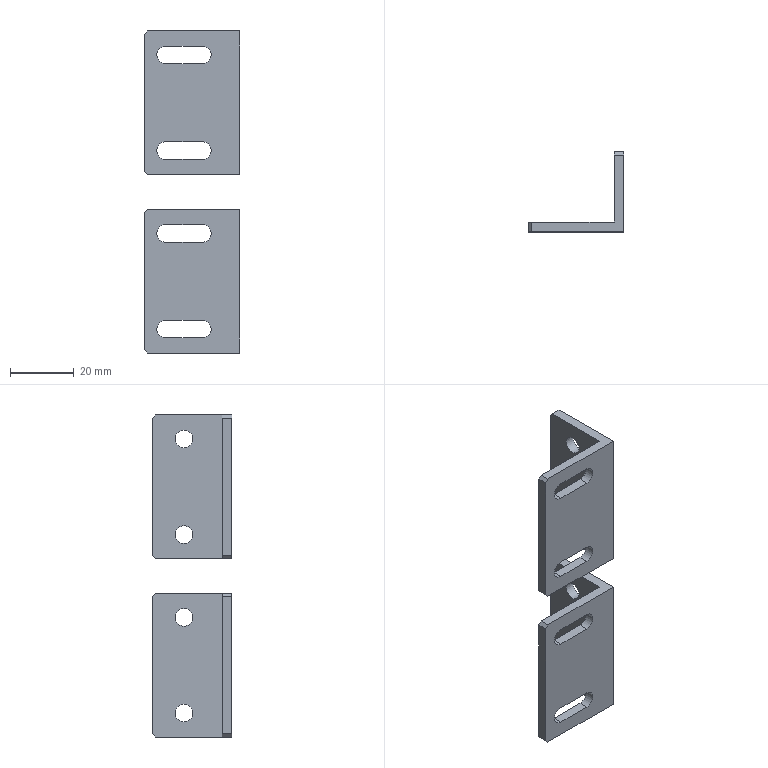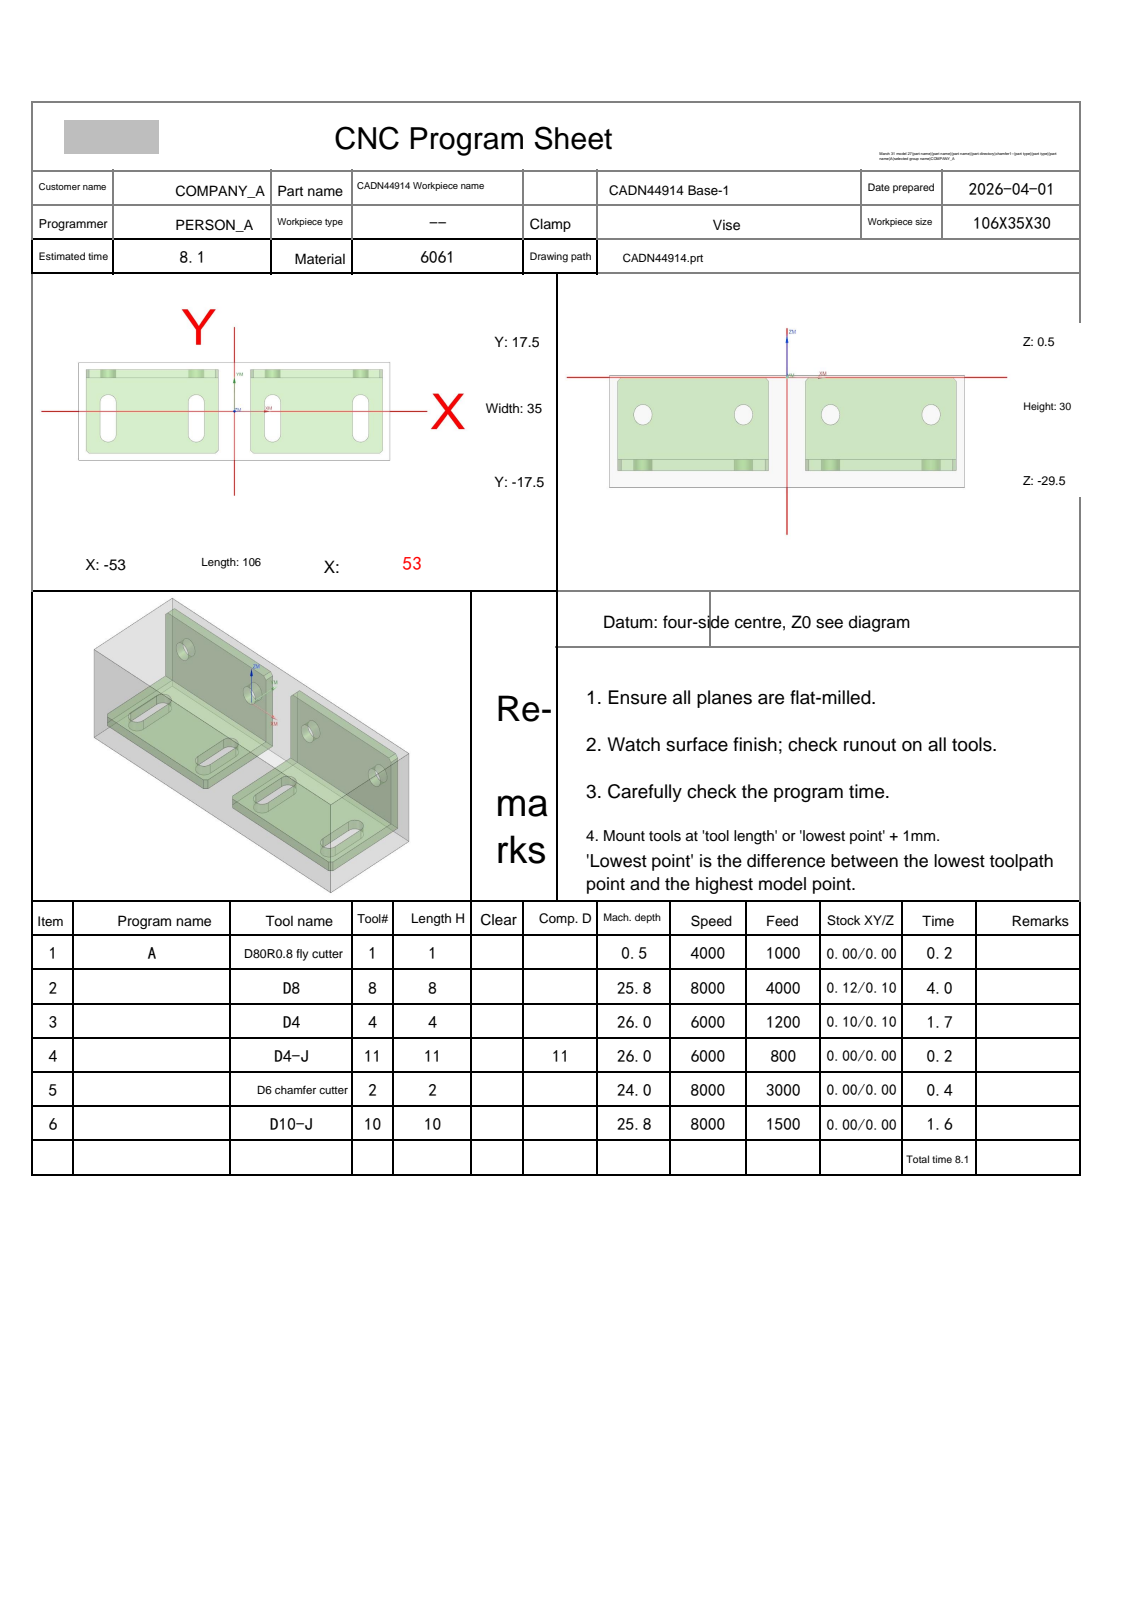NC program | NX | posted by the shop | part box 30 x 25 x 101 mm
Lines 33 to 938 of 5910:
N2 T08 M06
(D8  D=8. R=0. H=08 ce=0.12 di=0.10)
G00 G90 G54 X62.516 Y16.107 M03 S8000
G43 H08 Z20.
M08
Z-10.65
G01 X62.417 Y16.091 Z-11.275 F4000.
X62.318 Y16.075 Z-11.522
X62.219 Y16.059 Z-11.704
X62.121 Y16.043 Z-11.85
X62.022 Y16.027 Z-11.973
X61.923 Y16.011 Z-12.078
X61.825 Y15.995 Z-12.17
X61.726 Y15.979 Z-12.25
X61.627 Y15.963 Z-12.32
X61.529 Y15.947 Z-12.382
X61.43 Y15.931 Z-12.436
X61.331 Y15.915 Z-12.483
X61.232 Y15.899 Z-12.524
X61.134 Y15.883 Z-12.558
X61.035 Y15.867 Z-12.586
X60.936 Y15.851 Z-12.61
X60.838 Y15.835 Z-12.627
X60.739 Y15.819 Z-12.64
X60.64 Y15.803 Z-12.647
X60.541 Y15.787 Z-12.65
X58.872 Y15.515
G03 X58.558 Y15.255 I.069 J-.404
X58.044 Y11.824 I11.196 J-3.431
G01 Y11.754
G03 X57.949 Y3.73 I339.384 J-8.023
X57.95 Y2.791 I339.479 J0.0
G01 X57.931 Y-16.168
G02 X53.968 Y-21.494 I-5.735 J.13
X48.72 Y-22.354 I-5.366 J16.303
X40.208 Y-22.456 I-8.512 J354.954
X38.161 Y-22.45 I0.0 J355.056
G01 X-51.678 Y-22.43
G02 X-56.969 Y-18.509 I.136 J5.714
X-57.846 Y-13.325 I15.967 J5.368
X-57.953 Y-5.477 I289.574 J7.847
X-57.949 Y-4.086 I289.681 J0.0
G01 X-57.931 Y16.154
G02 X-54.076 Y21.44 I5.698 J-.107
X-48.897 Y22.342 I5.375 J-15.529
X-40.524 Y22.458 I8.373 J-302.172
X-38.219 Y22.45 I0.0 J-302.288
G01 X51.741 Y22.427
G02 X57.07 Y18.146 I-.192 J-5.697
X57.491 Y14.544 I-15.208 J-3.602
X57.463 Y13.62 I-15.628 J0.0
G03 X57.351 Y3.991 I606.655 J-11.894
G01 X57.332 Y-14.688
G02 X53.425 Y-20.418 I-6.439 J.194
X47.956 Y-21.66 I-6.092 J14.165
X40.512 Y-21.856 I-7.444 J140.749
X38.96 Y-21.848 I0.0 J140.945
G01 X-50.327 Y-21.825
G02 X-55.877 Y-17.993 I.331 J6.415
X-57.152 Y-12.533 I13.846 J6.11
X-57.358 Y-4.985 I137.85 J7.548
X-57.348 Y-3.297 I138.056 J0.0
G01 X-57.334 Y14.627
G02 X-53.521 Y20.363 I6.425 J-.136
X-47.945 Y21.659 I6.167 J-13.892
X-40.439 Y21.857 I7.506 J-141.907
X-38.829 Y21.848 I0.0 J-142.105
G01 X50.187 Y21.832
G02 X55.925 Y17.551 I-.143 J-6.177
X56.733 Y12.44 I-15.748 J-5.11
G01 Y12.296
G02 X56.763 Y5.932 I-660.189 J-6.364
X56.751 Y1.891 I-660.22 J0.0
X56.771 Y-3.975 I-877.532 J-5.866
X56.718 Y-13.548 I-877.551 J0.0
X52.464 Y-19.656 I-7.15 J.444
X46.419 Y-21.046 I-6.699 J15.305
X38.343 Y-21.259 I-8.076 J152.558
X36.463 Y-21.248 I0.0 J152.772
G01 X-48.937 Y-21.224
G02 X-55.152 Y-16.964 I.346 J7.169
X-56.53 Y-11.098 I15.026 J6.624
X-56.762 Y-2.879 I145.33 J8.219
X-56.748 Y-.843 I145.562 J0.0
X-56.767 Y4.609 I770.486 J5.452
X-56.715 Y13.577 I770.505 J0.0
X-52.493 Y19.637 I7.146 J-.478
X-46.749 Y21.017 I6.58 J-14.744
X-38.468 Y21.264 I8.281 J-138.804
X-36.375 Y21.248 I0.0 J-139.051
G01 X48.785 Y21.231
G02 X54.926 Y16.953 I-.153 J-6.766
X56.047 Y11.274 I-15.235 J-5.957
X56.174 Y1.718 I-357.138 J-9.556
X56.15 Y-2.427 I-357.266 J0.0
X56.174 Y-6.04 I-275.832 J-3.613
X56.099 Y-12.466 I-275.856 J0.0
X51.293 Y-19.07 I-7.778 J.609
X44.934 Y-20.447 I-7.048 J17.185
X36.468 Y-20.659 I-8.466 J168.493
X34.498 Y-20.648 I0.0 J168.706
G01 X-47.542 Y-20.626
G02 X-54.546 Y-15.835 I.2 J7.809
X-55.919 Y-9.777 I16.529 J6.929
X-56.163 Y-1.075 I154.575 J8.702
X-56.148 Y1.138 I154.819 J0.0
X-56.157 Y4.648 I663.047 J3.51
X-56.113 Y12.257 I663.056 J0.0
X-53.836 Y17.363 I7.476 J-.274
X-51.867 Y18.926 I3.623 J-2.541
X-45.235 Y20.432 I7.404 J-17.255
X-36.921 Y20.657 I8.314 J-153.529
X-35.159 Y20.647 I0.0 J-153.754
G01 X47.421 Y20.631
G02 X52.399 Y18.635 I-.044 J-7.317
X54.068 Y17.06 I-2.112 J-3.911
X55.259 Y12.19 I-13.92 J-5.984
X55.559 Y4.973 I-86.472 J-7.217
X55.547 Y3.499 I-86.773 J0.0
X55.566 Y-2.101 I-811.454 J-5.6
X55.518 Y-10.94 I-811.473 J0.0
X50.295 Y-18.445 I-8.318 J.219
X43.928 Y-19.823 I-7.236 J18.035
X35.476 Y-20.056 I-8.452 J153.016
X33.732 Y-20.046 I0.0 J153.249
G01 X-46.027 Y-20.034
X-46.181 Y-20.035
G02 X-53.946 Y-14.785 I0.0 J8.368
X-55.34 Y-8.184 I18.432 J7.341
X-55.554 Y.16 I162.754 J8.345
X-55.546 Y1.772 I162.968 J0.0
X-55.57 Y5.167 I243.213 J3.395
X-55.493 Y11.271 I243.237 J0.0
X-54.62 Y14.627 I10.704 J-.994
X-54.625 Y14.848 I4.478 J.221
X-53.413 Y17.913 I4.483 J0.0
X-50.498 Y19.12 I3.041 J-3.221
X-38.847 Y20.04 I11.651 J-73.341
X-37.813 Y20.032 I0.0 J-74.261
G01 X46.087 Y20.031
G02 X49.997 Y19.12 I-.377 J-10.464
X50.293 Y19.129 I.296 J-4.764
X52.453 Y18.612 I0.0 J-4.773
G03 X50.253 Y19.134 I-2.2 J-4.376
X49.877 Y19.12 I0.0 J-4.898
X42.529 Y19.577 I-7.348 J-58.761
X41.176 Y19.562 I0.0 J-59.218
G01 X-38.344 Y19.543
X-38.43
G03 X-46.798 Y19.12 I0.0 J-82.957
G01 X-50.498
X-5.206 Y19.099
G03 X2.028 Y18.963 I7.233 J191.611
X4.429 Y18.978 I0.0 J191.748
G01 X5.502 Y19.12
X49.902
G03 X50.302 Y19.52 I0.0 J.4
X50.116 Y19.857 I-.4 J0.0
G01 X49.518 Y20.237
X48.185 Y21.084 Z-12.55
X47.915 Y21.255
X47.866 Y21.282
X47.814 Y21.301
X47.759 Y21.313
X47.704 Y21.318
X5.983 Y21.67
X5.917 Y21.665
X5.852 Y21.648
X5.79 Y21.622
X5.734 Y21.585
X5.685 Y21.54
X5.644 Y21.487
X5.613 Y21.428
X5.478 Y21.116
X4.85 Y19.667 Z-12.65
X4.727 Y19.37
G02 X4.038 Y18.853 I-.713 J.232
X-.04 Y18.522 I-4.078 J24.962
X-.806 Y18.534 I0.0 J25.293
G01 X-3.48 Y18.584
G03 X-5.498 Y19.12 I-2.169 J-4.106
G02 X-3.387 Y18.54 I-.174 J-4.768
G03 X-.092 Y18.042 I3.295 J10.652
X.316 Y18.049 I0.0 J11.151
X.604 Y18.047 I.288 J17.386
X2.942 Y18.205 I0.0 J17.389
G02 X4.327 Y18.935 I2.618 J-3.285
G03 X2.916 Y18.173 I1.146 J-3.809
G02 X.092 Y17.684 I-2.824 J7.906
X-.583 Y17.711 I0.0 J8.396
X-2.733 Y18.025 I.065 J7.962
G01 X-3.44 Y18.568
G03 X-.35 Y17.337 I3.115 J3.325
X.324 Y17.304 I.674 J6.969
X2.291 Y17.586 I0.0 J7.002
G02 X2.968 Y18.205 I3.756 J-3.425
G03 X2.327 Y17.586 I1.262 J-1.946
G02 X.075 Y17.02 I-2.252 J4.193
X-.563 Y17.063 I0.0 J4.76
X-2.302 Y17.542 I.006 J3.412
G01 X-2.634 Y17.95
G03 X-.588 Y16.782 I2.21 J1.496
X.191 Y16.712 I.778 J4.275
X1.92 Y17.071 I0.0 J4.345
G01 X2.385 Y17.65
G02 X.59 Y16.541 I-1.891 J1.053
X-.018 Y16.491 I-.608 J3.719
X-1.862 Y16.973 I0.0 J3.769
G01 X-2.268 Y17.498
G03 X-.107 Y16.241 I2.161 J1.229
G01 X-.033 Y16.242
G03 X.291 Y16.221 I.324 J2.437
X1.776 Y16.72 I0.0 J2.458
G01 X1.932 Y17.06
G02 X.952 Y16.188 I-1.2 J.361
X.024 Y16.034 I-.928 J2.735
X-1.732 Y16.629 I0.0 J2.889
G01 X-1.932 Y17.06
G03 X-.503 Y15.885 I1.602 J.492
X.117 Y15.807 I.62 J2.416
X1.586 Y16.285 I0.0 J2.494
G01 X1.809 Y16.763
G02 X.631 Y15.724 I-1.342 J.335
X-.008 Y15.634 I-.639 J2.23
X-1.597 Y16.264 I0.0 J2.32
G01 X-1.773 Y16.676
G03 X-.166 Y15.461 I1.621 J.474
X.163 Y15.433 I.329 J1.919
X1.459 Y15.928 I0.0 J1.947
G01 X1.635 Y16.343
G02 X.509 Y15.351 I-1.257 J.292
X.006 Y15.291 I-.503 J2.051
X-1.45 Y15.873 I0.0 J2.112
G01 X-1.612 Y16.288
G03 X-.263 Y15.14 I1.426 J.309
X.141 Y15.091 I.404 J1.643
X1.456 Y15.718 I0.0 J1.692
G01 X1.52 Y16.066
G02 X.681 Y15.084 I-1.026 J.027
X.015 Y14.964 I-.666 J1.788
X-1.436 Y15.632 I0.0 J1.908
G01 X-1.51 Y15.99
G03 X-.594 Y14.908 I1.164 J.056
X.061 Y14.785 I.655 J1.688
X1.392 Y15.368 I0.0 J1.81
G01 X1.493 Y15.862
X1.494 Y15.834
G02 X.546 Y14.739 I-1.106 J0.0
X.009 Y14.657 I-.537 J1.711
X-1.403 Y15.344 I0.0 J1.793
G01 X-1.478 Y15.743
G03 X-.419 Y14.558 I1.224 J.029
X.085 Y14.479 I.504 J1.563
X1.376 Y15.106 I0.0 J1.642
G01 X1.452 Y15.549
X1.453 Y15.526
G02 X.494 Y14.431 I-1.105 J0.0
X-.016 Y14.349 I-.51 J1.538
X-1.388 Y15.107 I0.0 J1.621
G01 X-1.438 Y15.438
G03 X-.425 Y14.269 I1.205 J.021
X.067 Y14.194 I.492 J1.563
X1.334 Y14.794 I0.0 J1.639
G01 X1.412 Y15.239
Y15.205
G02 X.497 Y14.147 I-1.07 J0.0
X.004 Y14.071 I-.492 J1.556
X-1.351 Y14.794 I0.0 J1.632
G01 X-1.396 Y15.119
Y15.103
G03 X-.521 Y14.021 I1.106 J0.0
X.068 Y13.904 I.59 J1.428
X1.356 Y14.595 I0.0 J1.545
G01 X1.38 Y15.001
X1.391 Y14.861
G02 X.67 Y13.931 I-.961 J0.0
X.009 Y13.786 I-.661 J1.438
X-1.365 Y14.583 I0.0 J1.583
G01 X-1.38 Y14.906
X-1.385 Y14.804
G03 X-.551 Y13.755 I1.076 J0.0
X.057 Y13.633 I.609 J1.458
X1.349 Y14.304 I0.0 J1.58
G01 X1.381 Y14.678
X1.386 Y14.573
G02 X.685 Y13.661 I-.944 J0.0
X.014 Y13.512 I-.671 J1.437
X-1.365 Y14.314 I0.0 J1.586
G01 X-1.381 Y14.638
X-1.385 Y14.537
G03 X-.537 Y13.475 I1.088 J0.0
X.066 Y13.352 I.603 J1.414
X1.358 Y14.057 I0.0 J1.537
G01 X1.381 Y14.404
X1.386 Y14.305
G02 X.682 Y13.385 I-.953 J0.0
X.016 Y13.239 I-.667 J1.449
X-1.363 Y14.032 I0.0 J1.595
G01 X-1.381 Y14.364
X-1.386 Y14.261
G03 X-.565 Y13.211 I1.082 J0.0
X.057 Y13.081 I.622 J1.432
X1.355 Y13.775 I0.0 J1.561
G01 X1.381 Y14.198
X1.393 Y14.044
G02 X.699 Y13.118 I-.965 J0.0
X.018 Y12.967 I-.681 J1.465
X-1.356 Y13.733 I0.0 J1.616
G01 X-1.382 Y14.095
X-1.387 Y13.989
G03 X-.567 Y12.936 I1.086 J0.0
X.067 Y12.799 I.633 J1.393
X1.361 Y13.514 I0.0 J1.53
G01 X1.381 Y13.852
X1.387 Y13.752
G02 X.7 Y12.843 I-.944 J0.0
X.011 Y12.684 I-.689 J1.417
X-1.368 Y13.497 I0.0 J1.575
G01 X-1.382 Y13.815
X-1.387 Y13.711
G03 X-.567 Y12.661 I1.082 J0.0
X.053 Y12.536 I.619 J1.474
X1.344 Y13.193 I0.0 J1.599
G01 X1.382 Y13.58
X1.387 Y13.48
G02 X.682 Y12.561 I-.951 J0.0
X.015 Y12.416 I-.667 J1.455
X-1.362 Y13.201 I0.0 J1.6
G01 X-1.382 Y13.54
X-1.387 Y13.439
G03 X-.547 Y12.379 I1.088 J0.0
X.064 Y12.253 I.611 J1.412
X1.36 Y12.963 I0.0 J1.538
G01 X1.382 Y13.308
X1.387 Y13.21
G02 X.682 Y12.286 I-.957 J0.0
X.014 Y12.14 I-.667 J1.445
X-1.366 Y12.937 I0.0 J1.592
G01 X-1.383 Y13.267
X-1.388 Y13.162
G03 X-.566 Y12.111 I1.083 J0.0
X.052 Y11.987 I.619 J1.474
X1.346 Y12.647 I0.0 J1.598
G01 X1.382 Y13.091
X1.393 Y12.949
G02 X.682 Y12.012 I-.972 J0.0
X.014 Y11.866 I-.667 J1.452
X-1.364 Y12.655 I0.0 J1.598
G01 X-1.383 Y12.992
X-1.388 Y12.888
G03 X-.567 Y11.836 I1.084 J0.0
X.053 Y11.71 I.62 J1.461
X1.35 Y12.382 I0.0 J1.587
G01 X1.383 Y12.818
X1.393 Y12.675
G02 X.682 Y11.737 I-.973 J0.0
X.014 Y11.591 I-.668 J1.448
X-1.363 Y12.381 I0.0 J1.595
G01 X-1.384 Y12.721
X-1.389 Y12.614
G03 X-.582 Y11.567 I1.084 J0.0
X.063 Y11.425 I.644 J1.395
X1.362 Y12.142 I0.0 J1.536
G01 X1.383 Y12.542
X1.393 Y12.4
G02 X.685 Y11.462 I-.975 J0.0
X.015 Y11.315 I-.67 J1.452
X-1.365 Y12.106 I0.0 J1.599
G01 X-1.384 Y12.443
X-1.389 Y12.34
G03 X-.57 Y11.285 I1.09 J0.0
X.049 Y11.16 I.619 J1.482
X1.345 Y11.819 I0.0 J1.606
G01 X1.383 Y12.266
X1.392 Y12.132
G02 X.639 Y11.164 I-.998 J0.0
X.019 Y11.04 I-.62 J1.488
X-1.36 Y11.817 I0.0 J1.612
G01 X-1.385 Y12.178
X-1.39 Y12.067
G03 X-.582 Y11.014 I1.089 J0.0
X.062 Y10.871 I.644 J1.379
X1.376 Y11.625 I0.0 J1.522
G01 X1.383 Y12.011
X1.396 Y11.852
G02 X.653 Y10.894 I-.989 J0.0
X.015 Y10.759 I-.638 J1.451
X-1.38 Y11.591 I0.0 J1.585
G01 X-1.385 Y11.908
X-1.395 Y11.765
G03 X-.67 Y10.775 I1.039 J0.0
X.052 Y10.598 I.723 J1.39
X1.42 Y11.4 I0.0 J1.567
G01 X1.386 Y11.818
G02 X1.429 Y11.544 I-.848 J-.274
X.867 Y10.716 I-.891 J0.0
X.024 Y10.474 I-.843 J1.351
X-1.43 Y11.418 I0.0 J1.592
G01 X-1.397 Y11.73
G03 X-1.433 Y11.473 I.921 J-.257
X-.885 Y10.608 I.956 J0.0
X.042 Y10.319 I.927 J1.34
X1.466 Y11.156 I0.0 J1.63
X1.434 Y11.577 I-3.694 J-.073
G02 X1.477 Y11.299 I-.873 J-.278
X.915 Y10.453 I-.917 J0.0
X.03 Y10.199 I-.885 J1.41
X-1.47 Y11.144 I0.0 J1.664
G01 X-1.445 Y11.501
G03 X-1.481 Y11.234 I.953 J-.268
X-.949 Y10.356 I.99 J0.0
X.041 Y10.036 I.991 J1.373
X1.51 Y10.887 I0.0 J1.693
G01 X1.513 Y10.99
G03 X1.484 Y11.32 I-1.88 J0.0
G02 X1.524 Y11.047 I-.903 J-.273
X.967 Y10.186 I-.943 J0.0
X.032 Y9.907 I-.935 J1.428
X-1.525 Y10.914 I0.0 J1.707
G01 X-1.485 Y11.306
G03 X-1.531 Y10.994 I1.023 J-.311
X-.896 Y10.017 I1.069 J0.0
X.045 Y9.738 I.941 J1.447
X1.567 Y10.651 I0.0 J1.726
X1.522 Y11.127 I-3.127 J-.059
G02 X1.58 Y10.796 I-.912 J-.332
X1.052 Y9.932 I-.97 J0.0
X.033 Y9.607 I-1.019 J1.437
X-1.583 Y10.665 I0.0 J1.762
G01 X-1.539 Y11.042
G03 X-1.586 Y10.726 I1.038 J-.316
X-.951 Y9.738 I1.085 J0.0
X.046 Y9.434 I.997 J1.481
X1.621 Y10.379 I0.0 J1.786
X1.58 Y10.832 I-3.737 J-.111
G02 X1.635 Y10.513 I-.9 J-.32
X1.156 Y9.685 I-.955 J0.0
X.034 Y9.299 I-1.123 J1.44
X-1.639 Y10.392 I0.0 J1.826
G01 X-1.601 Y10.743
G03 X-1.637 Y10.461 I1.097 J-.282
X-.977 Y9.431 I1.133 J0.0
X.047 Y9.121 I1.025 J1.534
X1.686 Y10.117 I0.0 J1.845
G01 X1.714 Y10.294
G03 X1.626 Y10.597 I-.569 J0.0
G02 X1.73 Y10.21 I-.671 J-.387
X1.459 Y9.621 I-.775 J0.0
X.039 Y8.981 I-1.42 J1.255
X-1.695 Y10.11 I0.0 J1.895
G01 X-1.717 Y10.27
G02 X-1.637 Y10.566 I.593 J0.0
G03 X-1.746 Y10.147 I.755 J-.419
X-1.475 Y9.519 I.864 J0.0
X.043 Y8.804 I1.519 J1.255
X1.744 Y9.78 I0.0 J1.97
X1.826 Y10.093 I-.557 J.314
X1.678 Y10.503 I-.639 J0.0
G02 X1.841 Y9.99 I-.724 J-.513
X1.524 Y9.31 I-.888 J0.0
X.04 Y8.662 I-1.485 J1.376
X-1.735 Y9.713 I0.0 J2.024
X-1.825 Y10.055 I.605 J.343
X-1.702 Y10.451 I.696 J0.0
G03 X-1.858 Y9.921 I.817 J-.53
X-1.56 Y9.22 I.974 J0.0
X.046 Y8.468 I1.606 J1.34
X1.843 Y9.488 I0.0 J2.092
X1.946 Y9.862 I-.623 J.374
X1.766 Y10.341 I-.726 J0.0
G02 X1.966 Y9.757 I-.753 J-.584
X1.668 Y9.064 I-.953 J0.0
X.043 Y8.315 I-1.624 J1.387
X-1.865 Y9.492 I0.0 J2.136
X-1.948 Y9.833 I.66 J.341
X-1.793 Y10.287 I.743 J0.0
G03 X-1.979 Y9.677 I.91 J-.61
X-1.611 Y8.858 I1.096 J0.0
X.049 Y8.113 I1.66 J1.478
X1.974 Y9.226 I0.0 J2.223
X2.08 Y9.601 I-.613 J.375
X1.932 Y10.038 I-.719 J0.0
G02 X2.1 Y9.488 I-.812 J-.55
X1.818 Y8.8 I-.981 J0.0
X.049 Y7.946 I-1.769 J1.407
X-2.022 Y9.301 I0.0 J2.26
X-2.081 Y9.592 I.695 J.291
X-1.921 Y10.056 I.754 J0.0
G03 X-2.118 Y9.418 I.935 J-.638
X-1.799 Y8.63 I1.132 J0.0
X.051 Y7.74 I1.85 J1.476
X2.113 Y8.944 I0.0 J2.367
X2.222 Y9.34 I-.661 J.396
X2.045 Y9.831 I-.771 J0.0
G02 X2.245 Y9.221 I-.83 J-.611
X1.974 Y8.524 I-1.031 J0.0
X.048 Y7.568 I-1.927 J1.462
X-2.142 Y8.959 I0.0 J2.418
X-2.224 Y9.32 I.746 J.361
X-2.041 Y9.84 I.829 J0.0
G03 X-2.266 Y9.145 I.963 J-.695
X-1.95 Y8.338 I1.188 J0.0
X.053 Y7.345 I2.003 J1.525
X2.262 Y8.655 I0.0 J2.518
X2.378 Y9.067 I-.674 J.412
X2.171 Y9.601 I-.79 J0.0
G02 X2.417 Y8.957 I-.721 J-.644
X2.248 Y8.41 I-.967 J0.0
X.041 Y7.176 I-2.207 J1.356
X-2.261 Y8.579 I0.0 J2.59
X-2.383 Y9.019 I.734 J.44
X-2.214 Y9.529 I.856 J0.0
G03 X-2.449 Y8.88 I.778 J-.649
X-2.292 Y8.338 I1.013 J0.0
X.068 Y6.939 I2.361 J1.291
X2.407 Y8.299 I0.0 J2.69
X2.558 Y8.821 I-.825 J.523
X2.434 Y9.299 I-.977 J0.0
G01 X2.261 Y9.465
G02 X2.621 Y8.722 I-.586 J-.743
X2.491 Y8.244 I-.946 J0.0
X.059 Y6.747 I-2.433 J1.229
X-1.039 Y6.978 I0.0 J2.725
X-2.552 Y8.88 I.688 J2.1
G01 Y8.903
G02 X-2.248 Y9.472 I.685 J0.0
G03 X-2.651 Y8.646 I.644 J-.826
X-2.53 Y8.156 I1.047 J0.0
X.059 Y6.501 I2.589 J1.196
X1.116 Y6.704 I0.0 J2.852
X2.761 Y8.695 I-.636 J2.201
X2.415 Y9.317 I-.729 J0.0
G02 X2.839 Y8.494 I-.587 J-.823
X2.74 Y8.058 I-1.011 J0.0
X.127 Y6.312 I-2.614 J1.084
X-.37 Y6.356 I0.0 J2.83
X-2.746 Y8.412 I.215 J2.649
X-2.772 Y8.62 I.815 J.208
X-2.44 Y9.29 I.841 J0.0
G03 X-2.871 Y8.399 I.705 J-.89
X-2.768 Y7.927 I1.135 J0.0
X.026 Y6.05 I2.795 J1.141
X.766 Y6.142 I0.0 J3.019
X2.988 Y8.316 I-.394 J2.625
G01 X3. Y8.449
G03 X2.643 Y9.098 I-.769 J0.0
G02 X3.078 Y8.247 I-.614 J-.851
X3.008 Y7.869 I-1.05 J0.0
X.204 Y5.863 I-2.803 J.956
G01 X.104 Y5.865
X-.074 Y5.86
G02 X-2.94 Y7.955 I0.0 J3.009
X-3.009 Y8.321 I.942 J.366
X-2.625 Y9.114 I1.01 J0.0
G03 X-3.111 Y8.141 I.732 J-.973
X-3.023 Y7.688 I1.218 J0.0
X-.025 Y5.583 I2.999 J1.083
X.354 Y5.605 I0.0 J3.188
X3.209 Y7.822 I-.073 J3.041
X3.259 Y8.123 I-.871 J.302
X2.89 Y8.861 I-.922 J0.0
G02 X3.336 Y7.947 I-.713 J-.914
X3.241 Y7.487 I-1.159 J0.0
X.195 Y5.37 I-3.046 J1.134
X-.044 Y5.379 I0.0 J3.25
G01 X-.094
G02 X-3.185 Y7.647 I0.0 J3.241
X-3.246 Y8.043 I1.265 J.395
X-3.083 Y8.679 I1.325 J0.0
G01 X-2.866 Y8.885
G03 X-3.369 Y7.844 I.826 J-1.041
X-3.264 Y7.329 I1.329 J0.0
X-.051 Y5.09 I3.214 J1.187
G01 X.119 Y5.094
X.233 Y5.092
G03 X3.425 Y7.31 I0.0 J3.405
X3.528 Y7.806 I-1.136 J.496
X3.292 Y8.534 I-1.239 J0.0
G01 X3.134 Y8.627
G02 X3.604 Y7.873 I-.37 J-.753
G01 X3.598 Y7.772
G02 X1.749 Y5.233 I-2.932 J.193
X.071 Y4.845 I-1.679 J3.438
X-3.236 Y6.747 I0.0 J3.826
X-3.508 Y7.69 I1.498 J.943
X-3.31 Y8.503 I1.77 J0.0
G01 X-3.148 Y8.618
G03 X-3.636 Y7.791 I.456 J-.827
G01 X-3.63 Y7.684
G03 X-1.725 Y4.98 I3.091 J.154
X.087 Y4.544 I1.812 J3.551
X3.524 Y6.511 I0.0 J3.986
X3.802 Y7.502 I-1.621 J.991
X3.6 Y8.355 I-1.9 J0.0
G01 X3.217 Y8.586
G02 X3.914 Y7.621 I-.319 J-.965
G01 X3.907 Y7.505
G02 X1.97 Y4.766 I-3.178 J.193
X.079 Y4.312 I-1.891 J3.714
X-3.442 Y6.249 I0.0 J4.168
X-3.795 Y7.406 I1.718 J1.157
X-3.554 Y8.377 I2.072 J0.0
G01 X-3.224 Y8.58
G03 X-3.94 Y7.548 I.386 J-1.032
G01 X-3.939 Y7.499
G03 X-2.037 Y4.549 I3.298 J.038
X.082 Y4. I2.119 J3.817
X3.726 Y5.961 I0.0 J4.366
X4.125 Y7.237 I-1.84 J1.276
X3.915 Y8.183 I-2.239 J0.0
X3.452 Y8.47 I-1.292 J-1.568
G02 X4.256 Y7.36 I-.365 J-1.11
G01 X4.247 Y7.214
G02 X2.177 Y4.266 I-3.47 J.236
X.083 Y3.75 I-2.094 J3.989
X-3.754 Y5.893 I0.0 J4.506
X-4.12 Y7.134 I1.916 J1.24
X-3.837 Y8.235 I2.283 J0.0
G01 X-3.448 Y8.47
G03 X-4.293 Y7.246 I.465 J-1.224
G01 X-4.284 Y7.09
G03 X-2.123 Y3.976 I3.664 J.236
X.086 Y3.43 I2.21 J4.195
X4.018 Y5.521 I0.0 J4.741
X4.477 Y6.97 I-2.058 J1.449
X4.25 Y8.013 I-2.517 J0.0
X3.784 Y8.306 I-1.157 J-1.326
G02 X4.614 Y7.146 I-.395 J-1.159
G01 X4.611 Y7.059
G02 X2.579 Y3.843 I-3.695 J.084
X.094 Y3.166 I-2.485 J4.223
X-4.033 Y5.424 I0.0 J4.9
X-4.47 Y6.858 I2.132 J1.434
X-4.176 Y8.051 I2.569 J0.0
X-3.763 Y8.316 I1.173 J-1.376
G03 X-4.636 Y7.063 I.463 J-1.253
G01 Y7.052
X-4.638 Y6.935
G03 X-2.863 Y3.759 I3.73 J0.0
X.084 Y2.831 I2.948 J4.216
X4.368 Y5.127 I0.0 J5.144
X4.854 Y6.714 I-2.347 J1.587
X4.672 Y7.715 I-2.833 J0.0
X4.152 Y8.124 I-.697 J-.349
G02 X4.944 Y7.206 I-.267 J-1.03
X4.983 Y6.68 I-3.497 J-.527
X3.686 Y3.942 I-3.536 J0.0
X.105 Y2.564 I-3.581 J3.965
X-4.264 Y4.831 I0.0 J5.343
X-4.839 Y6.59 I2.403 J1.758
X-4.615 Y7.723 I2.977 J0.0
X-4.052 Y8.174 I.819 J-.444
G03 X-5.025 Y6.836 I.446 J-1.347
G01 X-5.029 Y6.654
G03 X-3.2 Y3.285 I4.016 J0.0
X.088 Y2.216 I3.288 J4.523
X4.638 Y4.557 I0.0 J5.592
X5.257 Y6.429 I-2.52 J1.872
X5.055 Y7.536 I-3.139 J0.0
X4.316 Y8.066 I-.739 J-.25
G01 X4.293
G02 X5.291 Y7.221 I-.027 J-1.043
X5.405 Y6.329 I-3.423 J-.892
X4.46 Y3.922 I-3.537 J0.0
X.104 Y1.937 I-4.356 J3.787
X-4.602 Y4.368 I0.0 J5.772
X-5.239 Y6.321 I2.677 J1.953
X-5.048 Y7.431 I3.314 J0.0
X-4.267 Y8.069 I.849 J-.243
G03 X-5.282 Y7.233 I.074 J-1.123
X-5.444 Y6.159 I3.464 J-1.073
X-4.557 Y3.783 I3.627 J0.0
X.104 Y1.578 I4.66 J3.824
X5.002 Y4.093 I0.0 J6.029
X5.689 Y6.18 I-2.828 J2.086
X5.506 Y7.296 I-3.514 J0.0
X4.57 Y8.023 I-.938 J-.242
G01 X4.578
G02 X5.66 Y7.222 I0.0 J-1.132
X5.861 Y6.031 I-3.432 J-1.191
X5.112 Y3.822 I-3.633 J0.0
X.1 Y1.29 I-5.012 J3.696
X-4.936 Y3.854 I0.0 J6.228
X-5.669 Y6.061 I2.955 J2.207
X-5.489 Y7.199 I3.688 J0.0
X-4.812 Y7.986 I1.28 J-.418
G01 X-4.515 Y8.031
G03 X-5.745 Y6.987 I.085 J-1.347
X-5.892 Y5.909 I3.887 J-1.078
X-4.858 Y3.212 I4.034 J0.0
X.106 Y.914 I4.964 J4.212
X5.413 Y3.653 I0.0 J6.51
X6.152 Y5.915 I-3.089 J2.262
X5.939 Y7.173 I-3.829 J0.0
X4.949 Y7.965 I-1.029 J-.271
G02 X6.08 Y7.153 I-.009 J-1.207
X6.343 Y5.759 I-3.568 J-1.394
X5.669 Y3.588 I-3.831 J0.0
X.122 Y.615 I-5.547 J3.688
X-2.021 Y.969 I0.0 J6.661
X-6.053 Y5.055 I1.571 J5.583
X-6.164 Y5.855 I2.806 J.8
X-5.474 Y7.74 I2.917 J0.0
X-4.851 Y7.985 I.623 J-.668
G01 X-4.819 Y7.984
G03 X-6.152 Y6.955 I.052 J-1.445
X-6.375 Y5.612 I3.944 J-1.342
X-5.532 Y3.1 I4.166 J0.0
X.125 Y.23 I5.657 J4.139
X3.245 Y.963 I0.0 J7.009
X6.633 Y5.331 I-2.313 J5.291
X6.677 Y5.823 I-2.733 J.492
X5.85 Y7.8 I-2.777 J0.0
X5.32 Y7.908 I-.671 J-1.938
G01 X5.365 Y7.909
G02 X6.515 Y7.117 I0.0 J-1.231
X6.853 Y5.5 I-3.695 J-1.616
X6.266 Y3.405 I-4.033 J0.0
X.208 Y-.066 I-6.058 J3.55
X-.665 Y-.012 I0.0 J7.021
X-6.318 Y4.005 I.495 J6.683
X-6.639 Y5.513 I3.382 J1.508
X-6.135 Y7.377 I3.703 J0.0
X-5.214 Y7.925 I.921 J-.5
G01 X-5.205
G03 X-6.563 Y6.961 I.026 J-1.475
X-6.885 Y5.334 I3.952 J-1.628
X-6.254 Y3.098 I4.274 J0.0
X.027 Y-.463 I6.28 J3.757
X1.094 Y-.385 I0.0 J7.318
X6.835 Y3.791 I-.682 J6.971
X7.184 Y5.398 I-3.527 J1.607
X6.666 Y7.334 I-3.876 J0.0
X5.776 Y7.891 I-.89 J-.432
G01 X5.63 Y7.88
X5.786 Y7.89
G02 X6.937 Y7.143 I0.0 J-1.261
X7.392 Y5.256 I-3.694 J-1.887
X6.96 Y3.413 I-4.148 J0.0
X.71 Y-.738 I-6.605 J3.165
X-.007 Y-.772 I-.717 J7.496
X-6.461 Y2.88 I0.0 J7.53
X-7.133 Y5.253 I3.853 J2.373
X-6.834 Y6.872 I4.525 J0.0
X-5.845 Y7.88 I1.558 J-.54
G01 X-5.545
X-5.66 Y7.885
G03 X-6.947 Y7.05 I0.0 J-1.41
X-7.424 Y5.071 I3.874 J-1.979
X-6.953 Y3.102 I4.35 J0.0
X-.411 Y-1.148 I6.828 J3.349
X.247 Y-1.176 I.658 J7.826
X7.067 Y2.783 I0.0 J7.854
X7.709 Y5.153 I-4.056 J2.37
X7.373 Y6.898 I-4.697 J0.0
X6.4 Y7.88 I-1.52 J-.532
G01 X6.04
X6.203 Y7.89
G02 X7.386 Y7.164 I0.0 J-1.327
X7.952 Y5.025 I-3.76 J-2.138
X7.605 Y3.327 I-4.326 J0.0
X1.568 Y-1.365 I-7.111 J2.919
X.049 Y-1.507 I-1.519 J8.068
X-6.766 Y2.125 I0.0 J8.21
X-7.666 Y5.026 I4.228 J2.901
X-7.446 Y6.509 I5.127 J0.0
X-6.285 Y7.873 I2.084 J-.599
G01 X-5.883 Y7.88
X-6.029 Y7.887
G03 X-7.452 Y6.978 I0.0 J-1.569
X-7.981 Y4.832 I4.084 J-2.145
X-7.565 Y2.918 I4.614 J0.0
X-1.268 Y-1.793 I7.324 J3.225
X.195 Y-1.919 I1.462 J8.443
X7.338 Y1.917 I0.0 J8.569
X8.266 Y4.935 I-4.443 J3.018
X8.018 Y6.547 I-5.37 J0.0
X6.927 Y7.869 I-2.126 J-.644
G01 X6.439 Y7.88
G02 X6.642 Y7.895 I.202 J-1.381
X7.854 Y7.19 I0.0 J-1.396
X8.535 Y4.819 I-3.79 J-2.371
X8.294 Y3.372 I-4.47 J0.0
X2.95 Y-1.792 I-7.568 J2.485
X.108 Y-2.256 I-2.843 J8.474
X-7.011 Y1.278 I0.0 J8.938
X-8.223 Y4.832 I4.606 J3.555
X-8.092 Y6.062 I5.818 J0.0
X-6.741 Y7.868 I2.556 J-.504
G01 X-6.25 Y7.88
X-6.448 Y7.892
G03 X-7.92 Y7.008 I0.0 J-1.667
X-8.563 Y4.6 I4.187 J-2.408
X-8.211 Y2.79 I4.83 J0.0
X-2.131 Y-2.387 I7.839 J3.047
X.167 Y-2.678 I2.298 J8.954
X7.758 Y1.29 I0.0 J9.244
X8.851 Y4.713 I-4.812 J3.423
X8.629 Y6.317 I-5.905 J0.0
X7.439 Y7.859 I-2.538 J-.727
G01 X6.86 Y7.88
G02 X7.085 Y7.897 I.225 J-1.517
X8.434 Y7.091 I0.0 J-1.534
X9.135 Y4.574 I-4.17 J-2.517
X8.851 Y2.935 I-4.871 J0.0
X3.178 Y-2.512 I-8.104 J2.763
X.11 Y-3.018 I-3.068 J9.05
X-7.49 Y.746 I0.0 J9.556
X-8.808 Y4.587 I4.94 J3.841
X-8.661 Y5.932 I6.257 J0.0
X-7.187 Y7.873 I2.717 J-.534
G01 X-6.725 Y7.88
X-6.915 Y7.891
G03 X-8.419 Y7.019 I0.0 J-1.734
X-9.166 Y4.383 I4.277 J-2.636
X-8.896 Y2.758 I5.024 J0.0
X-3.188 Y-2.874 I8.336 J2.741
X.143 Y-3.448 I3.332 J9.377
X8.108 Y.537 I0.0 J9.951
X9.457 Y4.528 I-5.226 J3.99
X9.312 Y5.9 I-6.575 J0.0
X7.966 Y7.853 I-2.978 J-.614
G01 X7.36 Y7.88
G02 X7.578 Y7.895 I.218 J-1.595
X8.988 Y7.062 I0.0 J-1.61
X9.758 Y4.362 I-4.35 J-2.7
X9.524 Y2.831 I-5.12 J0.0
X3.967 Y-3.047 I-8.624 J2.586
X.13 Y-3.792 I-3.837 J9.512
X-7.818 Y-.019 I0.0 J10.257
X-9.413 Y4.395 I5.31 J4.414
X-9.317 Y5.544 I6.906 J0.0
X-7.771 Y7.85 I3.258 J-.514
G01 X-7.16 Y7.88
G03 X-7.388 Y7.894 I-.227 J-1.826
X-8.987 Y6.964 I0.0 J-1.84
X-9.787 Y4.163 I4.504 J-2.8
X-9.559 Y2.626 I5.304 J0.0
X-4.027 Y-3.385 I8.837 J2.583
X.134 Y-4.231 I4.161 J9.799
X8.514 Y-.151 I0.0 J10.646
X10.086 Y4.327 I-5.592 J4.478
X9.971 Y5.605 I-7.164 J0.0
X8.513 Y7.848 I-3.336 J-.573
G01 X7.898 Y7.88
G02 X8.118 Y7.895 I.22 J-1.612
X9.518 Y7.097 I0.0 J-1.627
X10.401 Y4.169 I-4.415 J-2.928
X10.225 Y2.817 I-5.297 J0.0
X4.943 Y-3.475 I-9.113 J2.287
X.145 Y-4.581 I-4.798 J9.861
X-8.177 Y-.757 I0.0 J10.966
X-10.04 Y4.213 I5.696 J4.97
X-9.982 Y5.145 I7.56 J0.0
X-8.313 Y7.837 I3.615 J-.378
X-7.788 Y7.882 I.525 J-3.061
G01 X-7.675 Y7.88
G03 X-7.906 Y7.894 I-.231 J-1.876
X-9.522 Y6.984 I0.0 J-1.89
X-10.428 Y3.946 I4.639 J-3.038
X-10.23 Y2.479 I5.545 J0.0
X-4.708 Y-3.944 I9.363 J2.464
X.13 Y-5.026 I4.838 J10.277
X8.897 Y-.891 I0.0 J11.359
X10.737 Y4.156 I-6.002 J5.047
X10.665 Y5.214 I-7.842 J0.0
X9.109 Y7.826 I-3.758 J-.47
X8.595 Y7.891 I-.514 J-2.01
X8.385 Y7.88 I0.0 J-2.074
G02 X8.648 Y7.901 I.263 J-1.673
X10.065 Y7.135 I0.0 J-1.694
X11.061 Y3.989 I-4.466 J-3.146
X10.933 Y2.811 I-5.463 J0.0
X5.936 Y-3.851 I-9.581 J1.981
X.155 Y-5.384 I-5.781 J10.136
X-8.653 Y-1.37 I0.0 J11.669
X-10.686 Y4.01 I6.101 J5.38
X-10.642 Y4.852 I8.134 J0.0
X-9.086 Y7.702 I4.105 J-.392
X-8.393 Y7.901 I.693 J-1.106
X-8.158 Y7.88 I0.0 J-1.305
G03 X-8.406 Y7.895 I-.248 J-2.026
X-10.182 Y6.86 I0.0 J-2.041
X-11.084 Y3.719 I5.017 J-3.14
X-10.892 Y2.226 I5.919 J0.0
X-5.358 Y-4.516 I9.9 J2.485
X.13 Y-5.835 I5.487 J10.754
X9.383 Y-1.517 I0.0 J12.073
X11.405 Y3.976 I-6.449 J5.494
X11.357 Y4.883 I-8.471 J0.0
X9.709 Y7.811 I-4.083 J-.37
X9.195 Y7.898 I-.514 J-1.487
X8.961 Y7.88 I0.0 J-1.573
G02 X9.221 Y7.9 I.26 J-1.706
X10.654 Y7.137 I0.0 J-1.726
X11.736 Y3.814 I-4.555 J-3.322
X11.647 Y2.812 I-5.638 J0.0
X6.944 Y-4.177 I-10.032 J1.673
X.161 Y-6.196 I-6.783 J10.387
X-9.014 Y-2.14 I0.0 J12.405
X-11.353 Y3.845 I6.486 J5.985
X-11.335 Y4.401 I8.826 J0.0
X-9.761 Y7.622 I4.561 J-.235
X-8.947 Y7.901 I.814 J-1.047
X-8.711 Y7.88 I0.0 J-1.326
G03 X-8.965 Y7.896 I-.254 J-2.069